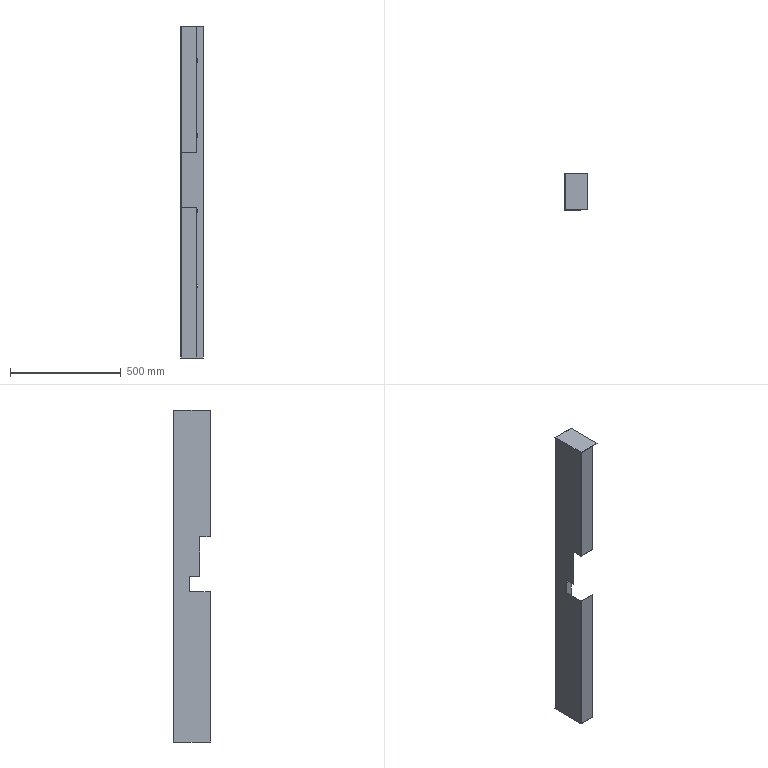Part | SolidWorks | features BaseBody 1 | 1 solid | 66 faces | box 103.5 x 169 x 1502 mm | volume 742622 mm3 | plane 42 | cylinder 24 | commonest cylinder face diameters 7 x16 1.473 x4 4.473 x4